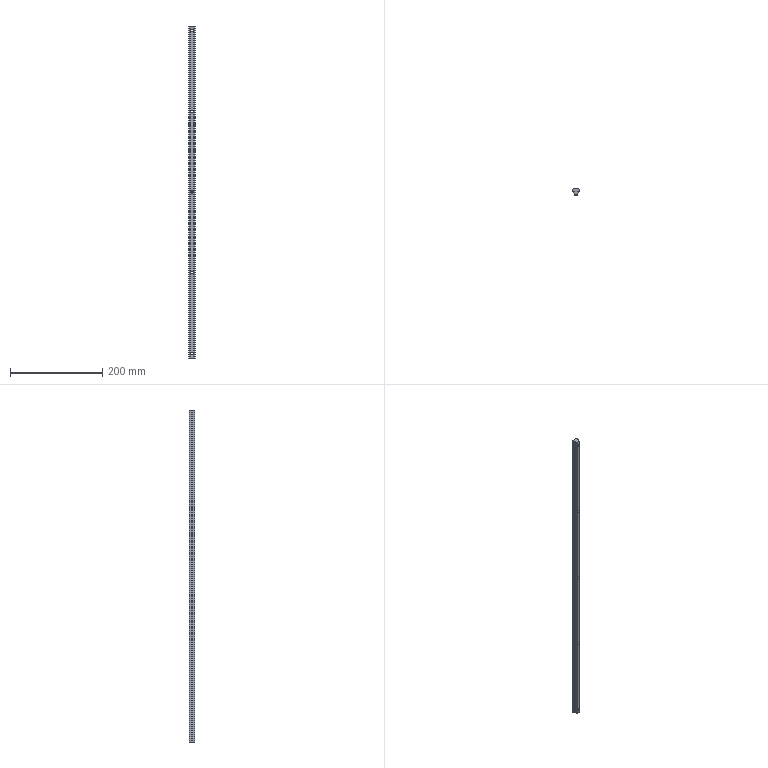Part | STEP file | TJ-DHQM-003-017 | 1 solid | 39 faces | box 15 x 13 x 720 mm | volume 103094 mm3 | cylinder 20 | plane 19 | commonest cylinder face diameters 5.5 x10 10 x10
STEP:
#1=CARTESIAN_POINT('',(0.,7.3,705.));
#2=VERTEX_POINT('',#1);
#3=CARTESIAN_POINT('',(0.,7.3,715.));
#4=VERTEX_POINT('',#3);
#5=CARTESIAN_POINT('',(0.,7.3,710.));
#6=DIRECTION('',(0.,1.,0.));
#7=DIRECTION('',(0.,0.,1.));
#8=AXIS2_PLACEMENT_3D('',#5,#6,#7);
#9=CIRCLE('',#8,5.);
#10=EDGE_CURVE('',#2,#4,#9,.T.);
#11=ORIENTED_EDGE('',*,*,#10,.F.);
#12=CARTESIAN_POINT('',(0.,13.,705.));
#13=VERTEX_POINT('',#12);
#14=CARTESIAN_POINT('',(0.,13.,705.));
#15=DIRECTION('',(0.,1.,0.));
#16=VECTOR('',#15,1000.);
#17=LINE('',#14,#16);
#18=EDGE_CURVE('',#2,#13,#17,.T.);
#19=ORIENTED_EDGE('',*,*,#18,.T.);
#20=CARTESIAN_POINT('',(0.,13.,715.));
#21=VERTEX_POINT('',#20);
#22=CARTESIAN_POINT('',(0.,13.,710.));
#23=DIRECTION('',(0.,1.,0.));
#24=DIRECTION('',(0.,0.,1.));
#25=AXIS2_PLACEMENT_3D('',#22,#23,#24);
#26=CIRCLE('',#25,5.);
#27=EDGE_CURVE('',#13,#21,#26,.T.);
#28=ORIENTED_EDGE('',*,*,#27,.T.);
#29=CARTESIAN_POINT('',(0.,13.,715.));
#30=DIRECTION('',(0.,1.,0.));
#31=VECTOR('',#30,1000.);
#32=LINE('',#29,#31);
#33=EDGE_CURVE('',#4,#21,#32,.T.);
#34=ORIENTED_EDGE('',*,*,#33,.F.);
#35=EDGE_LOOP('',(#11,#19,#28,#34));
#36=FACE_OUTER_BOUND('',#35,.T.);
#37=CARTESIAN_POINT('',(0.,13.,710.));
#38=DIRECTION('',(0.,1.,0.));
#39=DIRECTION('',(0.,0.,1.));
#40=AXIS2_PLACEMENT_3D('',#37,#38,#39);
#41=CYLINDRICAL_SURFACE('',#40,5.);
#42=ADVANCED_FACE('',(#36),#41,.F.);
#43=CARTESIAN_POINT('',(0.,0.,707.25));
#44=VERTEX_POINT('',#43);
#45=CARTESIAN_POINT('',(0.,0.,712.75));
#46=VERTEX_POINT('',#45);
#47=CARTESIAN_POINT('',(0.,0.,710.));
#48=DIRECTION('',(0.,1.,0.));
#49=DIRECTION('',(0.,0.,1.));
#50=AXIS2_PLACEMENT_3D('',#47,#48,#49);
#51=CIRCLE('',#50,2.75);
#52=EDGE_CURVE('',#44,#46,#51,.T.);
#53=ORIENTED_EDGE('',*,*,#52,.F.);
#54=CARTESIAN_POINT('',(0.,7.3,707.25));
#55=VERTEX_POINT('',#54);
#56=CARTESIAN_POINT('',(0.,13.,707.25));
#57=DIRECTION('',(0.,1.,0.));
#58=VECTOR('',#57,1000.);
#59=LINE('',#56,#58);
#60=EDGE_CURVE('',#44,#55,#59,.T.);
#61=ORIENTED_EDGE('',*,*,#60,.T.);
#62=CARTESIAN_POINT('',(0.,7.3,712.75));
#63=VERTEX_POINT('',#62);
#64=CARTESIAN_POINT('',(0.,7.3,710.));
#65=DIRECTION('',(0.,1.,0.));
#66=DIRECTION('',(0.,0.,1.));
#67=AXIS2_PLACEMENT_3D('',#64,#65,#66);
#68=CIRCLE('',#67,2.75);
#69=EDGE_CURVE('',#55,#63,#68,.T.);
#70=ORIENTED_EDGE('',*,*,#69,.T.);
#71=CARTESIAN_POINT('',(0.,13.,712.75));
#72=DIRECTION('',(0.,1.,0.));
#73=VECTOR('',#72,1000.);
#74=LINE('',#71,#73);
#75=EDGE_CURVE('',#46,#63,#74,.T.);
#76=ORIENTED_EDGE('',*,*,#75,.F.);
#77=EDGE_LOOP('',(#53,#61,#70,#76));
#78=FACE_OUTER_BOUND('',#77,.T.);
#79=CARTESIAN_POINT('',(0.,13.,710.));
#80=DIRECTION('',(0.,1.,0.));
#81=DIRECTION('',(0.,0.,1.));
#82=AXIS2_PLACEMENT_3D('',#79,#80,#81);
#83=CYLINDRICAL_SURFACE('',#82,2.75);
#84=ADVANCED_FACE('',(#78),#83,.F.);
#85=CARTESIAN_POINT('',(0.,7.3,355.));
#86=VERTEX_POINT('',#85);
#87=CARTESIAN_POINT('',(0.,7.3,365.));
#88=VERTEX_POINT('',#87);
#89=CARTESIAN_POINT('',(0.,7.3,360.));
#90=DIRECTION('',(0.,1.,0.));
#91=DIRECTION('',(0.,0.,1.));
#92=AXIS2_PLACEMENT_3D('',#89,#90,#91);
#93=CIRCLE('',#92,5.);
#94=EDGE_CURVE('',#86,#88,#93,.T.);
#95=ORIENTED_EDGE('',*,*,#94,.F.);
#96=CARTESIAN_POINT('',(0.,13.,355.));
#97=VERTEX_POINT('',#96);
#98=CARTESIAN_POINT('',(0.,13.,355.));
#99=DIRECTION('',(0.,1.,0.));
#100=VECTOR('',#99,1000.);
#101=LINE('',#98,#100);
#102=EDGE_CURVE('',#86,#97,#101,.T.);
#103=ORIENTED_EDGE('',*,*,#102,.T.);
#104=CARTESIAN_POINT('',(0.,13.,365.));
#105=VERTEX_POINT('',#104);
#106=CARTESIAN_POINT('',(0.,13.,360.));
#107=DIRECTION('',(0.,1.,0.));
#108=DIRECTION('',(0.,0.,1.));
#109=AXIS2_PLACEMENT_3D('',#106,#107,#108);
#110=CIRCLE('',#109,5.);
#111=EDGE_CURVE('',#97,#105,#110,.T.);
#112=ORIENTED_EDGE('',*,*,#111,.T.);
#113=CARTESIAN_POINT('',(0.,13.,365.));
#114=DIRECTION('',(0.,1.,0.));
#115=VECTOR('',#114,1000.);
#116=LINE('',#113,#115);
#117=EDGE_CURVE('',#88,#105,#116,.T.);
#118=ORIENTED_EDGE('',*,*,#117,.F.);
#119=EDGE_LOOP('',(#95,#103,#112,#118));
#120=FACE_OUTER_BOUND('',#119,.T.);
#121=CARTESIAN_POINT('',(0.,13.,360.));
#122=DIRECTION('',(0.,1.,0.));
#123=DIRECTION('',(0.,0.,1.));
#124=AXIS2_PLACEMENT_3D('',#121,#122,#123);
#125=CYLINDRICAL_SURFACE('',#124,5.);
#126=ADVANCED_FACE('',(#120),#125,.F.);
#127=CARTESIAN_POINT('',(0.,0.,357.25));
#128=VERTEX_POINT('',#127);
#129=CARTESIAN_POINT('',(0.,0.,362.75));
#130=VERTEX_POINT('',#129);
#131=CARTESIAN_POINT('',(0.,0.,360.));
#132=DIRECTION('',(0.,1.,0.));
#133=DIRECTION('',(0.,0.,1.));
#134=AXIS2_PLACEMENT_3D('',#131,#132,#133);
#135=CIRCLE('',#134,2.75);
#136=EDGE_CURVE('',#128,#130,#135,.T.);
#137=ORIENTED_EDGE('',*,*,#136,.F.);
#138=CARTESIAN_POINT('',(0.,7.3,357.25));
#139=VERTEX_POINT('',#138);
#140=CARTESIAN_POINT('',(0.,13.,357.25));
#141=DIRECTION('',(0.,1.,0.));
#142=VECTOR('',#141,1000.);
#143=LINE('',#140,#142);
#144=EDGE_CURVE('',#128,#139,#143,.T.);
#145=ORIENTED_EDGE('',*,*,#144,.T.);
#146=CARTESIAN_POINT('',(0.,7.3,362.75));
#147=VERTEX_POINT('',#146);
#148=CARTESIAN_POINT('',(0.,7.3,360.));
#149=DIRECTION('',(0.,1.,0.));
#150=DIRECTION('',(0.,0.,1.));
#151=AXIS2_PLACEMENT_3D('',#148,#149,#150);
#152=CIRCLE('',#151,2.75);
#153=EDGE_CURVE('',#139,#147,#152,.T.);
#154=ORIENTED_EDGE('',*,*,#153,.T.);
#155=CARTESIAN_POINT('',(0.,13.,362.75));
#156=DIRECTION('',(0.,1.,0.));
#157=VECTOR('',#156,1000.);
#158=LINE('',#155,#157);
#159=EDGE_CURVE('',#130,#147,#158,.T.);
#160=ORIENTED_EDGE('',*,*,#159,.F.);
#161=EDGE_LOOP('',(#137,#145,#154,#160));
#162=FACE_OUTER_BOUND('',#161,.T.);
#163=CARTESIAN_POINT('',(0.,13.,360.));
#164=DIRECTION('',(0.,1.,0.));
#165=DIRECTION('',(0.,0.,1.));
#166=AXIS2_PLACEMENT_3D('',#163,#164,#165);
#167=CYLINDRICAL_SURFACE('',#166,2.75);
#168=ADVANCED_FACE('',(#162),#167,.F.);
#169=CARTESIAN_POINT('',(0.,7.3,530.));
#170=VERTEX_POINT('',#169);
#171=CARTESIAN_POINT('',(0.,7.3,540.));
#172=VERTEX_POINT('',#171);
#173=CARTESIAN_POINT('',(0.,7.3,535.));
#174=DIRECTION('',(0.,1.,0.));
#175=DIRECTION('',(0.,0.,1.));
#176=AXIS2_PLACEMENT_3D('',#173,#174,#175);
#177=CIRCLE('',#176,5.);
#178=EDGE_CURVE('',#170,#172,#177,.T.);
#179=ORIENTED_EDGE('',*,*,#178,.F.);
#180=CARTESIAN_POINT('',(0.,13.,530.));
#181=VERTEX_POINT('',#180);
#182=CARTESIAN_POINT('',(0.,13.,530.));
#183=DIRECTION('',(0.,1.,0.));
#184=VECTOR('',#183,1000.);
#185=LINE('',#182,#184);
#186=EDGE_CURVE('',#170,#181,#185,.T.);
#187=ORIENTED_EDGE('',*,*,#186,.T.);
#188=CARTESIAN_POINT('',(0.,13.,540.));
#189=VERTEX_POINT('',#188);
#190=CARTESIAN_POINT('',(0.,13.,535.));
#191=DIRECTION('',(0.,1.,0.));
#192=DIRECTION('',(0.,0.,1.));
#193=AXIS2_PLACEMENT_3D('',#190,#191,#192);
#194=CIRCLE('',#193,5.);
#195=EDGE_CURVE('',#181,#189,#194,.T.);
#196=ORIENTED_EDGE('',*,*,#195,.T.);
#197=CARTESIAN_POINT('',(0.,13.,540.));
#198=DIRECTION('',(0.,1.,0.));
#199=VECTOR('',#198,1000.);
#200=LINE('',#197,#199);
#201=EDGE_CURVE('',#172,#189,#200,.T.);
#202=ORIENTED_EDGE('',*,*,#201,.F.);
#203=EDGE_LOOP('',(#179,#187,#196,#202));
#204=FACE_OUTER_BOUND('',#203,.T.);
#205=CARTESIAN_POINT('',(0.,13.,535.));
#206=DIRECTION('',(0.,1.,0.));
#207=DIRECTION('',(0.,0.,1.));
#208=AXIS2_PLACEMENT_3D('',#205,#206,#207);
#209=CYLINDRICAL_SURFACE('',#208,5.);
#210=ADVANCED_FACE('',(#204),#209,.F.);
#211=CARTESIAN_POINT('',(0.,0.,532.25));
#212=VERTEX_POINT('',#211);
#213=CARTESIAN_POINT('',(0.,0.,537.75));
#214=VERTEX_POINT('',#213);
#215=CARTESIAN_POINT('',(0.,0.,535.));
#216=DIRECTION('',(0.,1.,0.));
#217=DIRECTION('',(0.,0.,1.));
#218=AXIS2_PLACEMENT_3D('',#215,#216,#217);
#219=CIRCLE('',#218,2.75);
#220=EDGE_CURVE('',#212,#214,#219,.T.);
#221=ORIENTED_EDGE('',*,*,#220,.F.);
#222=CARTESIAN_POINT('',(0.,7.3,532.25));
#223=VERTEX_POINT('',#222);
#224=CARTESIAN_POINT('',(0.,13.,532.25));
#225=DIRECTION('',(0.,1.,0.));
#226=VECTOR('',#225,1000.);
#227=LINE('',#224,#226);
#228=EDGE_CURVE('',#212,#223,#227,.T.);
#229=ORIENTED_EDGE('',*,*,#228,.T.);
#230=CARTESIAN_POINT('',(0.,7.3,537.75));
#231=VERTEX_POINT('',#230);
#232=CARTESIAN_POINT('',(0.,7.3,535.));
#233=DIRECTION('',(0.,1.,0.));
#234=DIRECTION('',(0.,0.,1.));
#235=AXIS2_PLACEMENT_3D('',#232,#233,#234);
#236=CIRCLE('',#235,2.75);
#237=EDGE_CURVE('',#223,#231,#236,.T.);
#238=ORIENTED_EDGE('',*,*,#237,.T.);
#239=CARTESIAN_POINT('',(0.,13.,537.75));
#240=DIRECTION('',(0.,1.,0.));
#241=VECTOR('',#240,1000.);
#242=LINE('',#239,#241);
#243=EDGE_CURVE('',#214,#231,#242,.T.);
#244=ORIENTED_EDGE('',*,*,#243,.F.);
#245=EDGE_LOOP('',(#221,#229,#238,#244));
#246=FACE_OUTER_BOUND('',#245,.T.);
#247=CARTESIAN_POINT('',(0.,13.,535.));
#248=DIRECTION('',(0.,1.,0.));
#249=DIRECTION('',(0.,0.,1.));
#250=AXIS2_PLACEMENT_3D('',#247,#248,#249);
#251=CYLINDRICAL_SURFACE('',#250,2.75);
#252=ADVANCED_FACE('',(#246),#251,.F.);
#253=CARTESIAN_POINT('',(0.,7.3,180.));
#254=VERTEX_POINT('',#253);
#255=CARTESIAN_POINT('',(0.,7.3,190.));
#256=VERTEX_POINT('',#255);
#257=CARTESIAN_POINT('',(0.,7.3,185.));
#258=DIRECTION('',(0.,1.,0.));
#259=DIRECTION('',(0.,0.,1.));
#260=AXIS2_PLACEMENT_3D('',#257,#258,#259);
#261=CIRCLE('',#260,5.);
#262=EDGE_CURVE('',#254,#256,#261,.T.);
#263=ORIENTED_EDGE('',*,*,#262,.F.);
#264=CARTESIAN_POINT('',(0.,13.,180.));
#265=VERTEX_POINT('',#264);
#266=CARTESIAN_POINT('',(0.,13.,180.));
#267=DIRECTION('',(0.,1.,0.));
#268=VECTOR('',#267,1000.);
#269=LINE('',#266,#268);
#270=EDGE_CURVE('',#254,#265,#269,.T.);
#271=ORIENTED_EDGE('',*,*,#270,.T.);
#272=CARTESIAN_POINT('',(0.,13.,190.));
#273=VERTEX_POINT('',#272);
#274=CARTESIAN_POINT('',(0.,13.,185.));
#275=DIRECTION('',(0.,1.,0.));
#276=DIRECTION('',(0.,0.,1.));
#277=AXIS2_PLACEMENT_3D('',#274,#275,#276);
#278=CIRCLE('',#277,5.);
#279=EDGE_CURVE('',#265,#273,#278,.T.);
#280=ORIENTED_EDGE('',*,*,#279,.T.);
#281=CARTESIAN_POINT('',(0.,13.,190.));
#282=DIRECTION('',(0.,1.,0.));
#283=VECTOR('',#282,1000.);
#284=LINE('',#281,#283);
#285=EDGE_CURVE('',#256,#273,#284,.T.);
#286=ORIENTED_EDGE('',*,*,#285,.F.);
#287=EDGE_LOOP('',(#263,#271,#280,#286));
#288=FACE_OUTER_BOUND('',#287,.T.);
#289=CARTESIAN_POINT('',(0.,13.,185.));
#290=DIRECTION('',(0.,1.,0.));
#291=DIRECTION('',(0.,0.,1.));
#292=AXIS2_PLACEMENT_3D('',#289,#290,#291);
#293=CYLINDRICAL_SURFACE('',#292,5.);
#294=ADVANCED_FACE('',(#288),#293,.F.);
#295=CARTESIAN_POINT('',(0.,0.,182.25));
#296=VERTEX_POINT('',#295);
#297=CARTESIAN_POINT('',(0.,0.,187.75));
#298=VERTEX_POINT('',#297);
#299=CARTESIAN_POINT('',(0.,0.,185.));
#300=DIRECTION('',(0.,1.,0.));
#301=DIRECTION('',(0.,0.,1.));
#302=AXIS2_PLACEMENT_3D('',#299,#300,#301);
#303=CIRCLE('',#302,2.75);
#304=EDGE_CURVE('',#296,#298,#303,.T.);
#305=ORIENTED_EDGE('',*,*,#304,.F.);
#306=CARTESIAN_POINT('',(0.,7.3,182.25));
#307=VERTEX_POINT('',#306);
#308=CARTESIAN_POINT('',(0.,13.,182.25));
#309=DIRECTION('',(0.,1.,0.));
#310=VECTOR('',#309,1000.);
#311=LINE('',#308,#310);
#312=EDGE_CURVE('',#296,#307,#311,.T.);
#313=ORIENTED_EDGE('',*,*,#312,.T.);
#314=CARTESIAN_POINT('',(0.,7.3,187.75));
#315=VERTEX_POINT('',#314);
#316=CARTESIAN_POINT('',(0.,7.3,185.));
#317=DIRECTION('',(0.,1.,0.));
#318=DIRECTION('',(0.,0.,1.));
#319=AXIS2_PLACEMENT_3D('',#316,#317,#318);
#320=CIRCLE('',#319,2.75);
#321=EDGE_CURVE('',#307,#315,#320,.T.);
#322=ORIENTED_EDGE('',*,*,#321,.T.);
#323=CARTESIAN_POINT('',(0.,13.,187.75));
#324=DIRECTION('',(0.,1.,0.));
#325=VECTOR('',#324,1000.);
#326=LINE('',#323,#325);
#327=EDGE_CURVE('',#298,#315,#326,.T.);
#328=ORIENTED_EDGE('',*,*,#327,.F.);
#329=EDGE_LOOP('',(#305,#313,#322,#328));
#330=FACE_OUTER_BOUND('',#329,.T.);
#331=CARTESIAN_POINT('',(0.,13.,185.));
#332=DIRECTION('',(0.,1.,0.));
#333=DIRECTION('',(0.,0.,1.));
#334=AXIS2_PLACEMENT_3D('',#331,#332,#333);
#335=CYLINDRICAL_SURFACE('',#334,2.75);
#336=ADVANCED_FACE('',(#330),#335,.F.);
#337=CARTESIAN_POINT('',(0.,7.3,5.));
#338=VERTEX_POINT('',#337);
#339=CARTESIAN_POINT('',(0.,7.3,15.));
#340=VERTEX_POINT('',#339);
#341=CARTESIAN_POINT('',(0.,7.3,10.));
#342=DIRECTION('',(0.,1.,0.));
#343=DIRECTION('',(0.,0.,1.));
#344=AXIS2_PLACEMENT_3D('',#341,#342,#343);
#345=CIRCLE('',#344,5.);
#346=EDGE_CURVE('',#338,#340,#345,.T.);
#347=ORIENTED_EDGE('',*,*,#346,.F.);
#348=CARTESIAN_POINT('',(0.,13.,5.));
#349=VERTEX_POINT('',#348);
#350=CARTESIAN_POINT('',(0.,13.,5.));
#351=DIRECTION('',(0.,1.,0.));
#352=VECTOR('',#351,1000.);
#353=LINE('',#350,#352);
#354=EDGE_CURVE('',#338,#349,#353,.T.);
#355=ORIENTED_EDGE('',*,*,#354,.T.);
#356=CARTESIAN_POINT('',(0.,13.,15.));
#357=VERTEX_POINT('',#356);
#358=CARTESIAN_POINT('',(0.,13.,10.));
#359=DIRECTION('',(0.,1.,0.));
#360=DIRECTION('',(0.,0.,1.));
#361=AXIS2_PLACEMENT_3D('',#358,#359,#360);
#362=CIRCLE('',#361,5.);
#363=EDGE_CURVE('',#349,#357,#362,.T.);
#364=ORIENTED_EDGE('',*,*,#363,.T.);
#365=CARTESIAN_POINT('',(0.,13.,15.));
#366=DIRECTION('',(0.,1.,0.));
#367=VECTOR('',#366,1000.);
#368=LINE('',#365,#367);
#369=EDGE_CURVE('',#340,#357,#368,.T.);
#370=ORIENTED_EDGE('',*,*,#369,.F.);
#371=EDGE_LOOP('',(#347,#355,#364,#370));
#372=FACE_OUTER_BOUND('',#371,.T.);
#373=CARTESIAN_POINT('',(0.,13.,10.));
#374=DIRECTION('',(0.,1.,0.));
#375=DIRECTION('',(0.,0.,1.));
#376=AXIS2_PLACEMENT_3D('',#373,#374,#375);
#377=CYLINDRICAL_SURFACE('',#376,5.);
#378=ADVANCED_FACE('',(#372),#377,.F.);
#379=CARTESIAN_POINT('',(0.,0.,7.25));
#380=VERTEX_POINT('',#379);
#381=CARTESIAN_POINT('',(0.,0.,12.75));
#382=VERTEX_POINT('',#381);
#383=CARTESIAN_POINT('',(0.,0.,10.));
#384=DIRECTION('',(0.,1.,0.));
#385=DIRECTION('',(0.,0.,1.));
#386=AXIS2_PLACEMENT_3D('',#383,#384,#385);
#387=CIRCLE('',#386,2.75);
#388=EDGE_CURVE('',#380,#382,#387,.T.);
#389=ORIENTED_EDGE('',*,*,#388,.F.);
#390=CARTESIAN_POINT('',(0.,7.3,7.25));
#391=VERTEX_POINT('',#390);
#392=CARTESIAN_POINT('',(0.,13.,7.25));
#393=DIRECTION('',(0.,1.,0.));
#394=VECTOR('',#393,1000.);
#395=LINE('',#392,#394);
#396=EDGE_CURVE('',#380,#391,#395,.T.);
#397=ORIENTED_EDGE('',*,*,#396,.T.);
#398=CARTESIAN_POINT('',(0.,7.3,12.75));
#399=VERTEX_POINT('',#398);
#400=CARTESIAN_POINT('',(0.,7.3,10.));
#401=DIRECTION('',(0.,1.,0.));
#402=DIRECTION('',(0.,0.,1.));
#403=AXIS2_PLACEMENT_3D('',#400,#401,#402);
#404=CIRCLE('',#403,2.75);
#405=EDGE_CURVE('',#391,#399,#404,.T.);
#406=ORIENTED_EDGE('',*,*,#405,.T.);
#407=CARTESIAN_POINT('',(0.,13.,12.75));
#408=DIRECTION('',(0.,1.,0.));
#409=VECTOR('',#408,1000.);
#410=LINE('',#407,#409);
#411=EDGE_CURVE('',#382,#399,#410,.T.);
#412=ORIENTED_EDGE('',*,*,#411,.F.);
#413=EDGE_LOOP('',(#389,#397,#406,#412));
#414=FACE_OUTER_BOUND('',#413,.T.);
#415=CARTESIAN_POINT('',(0.,13.,10.));
#416=DIRECTION('',(0.,1.,0.));
#417=DIRECTION('',(0.,0.,1.));
#418=AXIS2_PLACEMENT_3D('',#415,#416,#417);
#419=CYLINDRICAL_SURFACE('',#418,2.75);
#420=ADVANCED_FACE('',(#414),#419,.F.);
#421=CARTESIAN_POINT('',(7.5,7.5,720.));
#422=VERTEX_POINT('',#421);
#423=CARTESIAN_POINT('',(7.5,12.,720.));
#424=VERTEX_POINT('',#423);
#425=CARTESIAN_POINT('',(7.5,13.,720.));
#426=DIRECTION('',(0.,1.,0.));
#427=VECTOR('',#426,1000.);
#428=LINE('',#425,#427);
#429=EDGE_CURVE('',#422,#424,#428,.T.);
#430=ORIENTED_EDGE('',*,*,#429,.F.);
#431=CARTESIAN_POINT('',(7.5,7.5,0.));
#432=VERTEX_POINT('',#431);
#433=CARTESIAN_POINT('',(7.5,7.5,720.));
#434=DIRECTION('',(0.,0.,-1.));
#435=VECTOR('',#434,1000.);
#436=LINE('',#433,#435);
#437=EDGE_CURVE('',#422,#432,#436,.T.);
#438=ORIENTED_EDGE('',*,*,#437,.T.);
#439=CARTESIAN_POINT('',(7.5,12.,0.));
#440=VERTEX_POINT('',#439);
#441=CARTESIAN_POINT('',(7.5,13.,0.));
#442=DIRECTION('',(0.,1.,0.));
#443=VECTOR('',#442,1000.);
#444=LINE('',#441,#443);
#445=EDGE_CURVE('',#432,#440,#444,.T.);
#446=ORIENTED_EDGE('',*,*,#445,.T.);
#447=CARTESIAN_POINT('',(7.5,12.,720.));
#448=DIRECTION('',(0.,0.,1.));
#449=VECTOR('',#448,1000.);
#450=LINE('',#447,#449);
#451=EDGE_CURVE('',#440,#424,#450,.T.);
#452=ORIENTED_EDGE('',*,*,#451,.T.);
#453=EDGE_LOOP('',(#430,#438,#446,#452));
#454=FACE_OUTER_BOUND('',#453,.T.);
#455=CARTESIAN_POINT('',(7.5,13.,720.));
#456=DIRECTION('',(-1.,0.,0.));
#457=DIRECTION('',(0.,-1.,0.));
#458=AXIS2_PLACEMENT_3D('',#455,#456,#457);
#459=PLANE('',#458);
#460=ADVANCED_FACE('',(#454),#459,.F.);
#461=CARTESIAN_POINT('',(0.,13.,710.));
#462=DIRECTION('',(0.,1.,0.));
#463=DIRECTION('',(0.,0.,1.));
#464=AXIS2_PLACEMENT_3D('',#461,#462,#463);
#465=CIRCLE('',#464,5.);
#466=EDGE_CURVE('',#21,#13,#465,.T.);
#467=ORIENTED_EDGE('',*,*,#466,.F.);
#468=ORIENTED_EDGE('',*,*,#27,.F.);
#469=EDGE_LOOP('',(#467,#468));
#470=FACE_BOUND('',#469,.T.);
#471=CARTESIAN_POINT('',(0.,13.,360.));
#472=DIRECTION('',(0.,1.,0.));
#473=DIRECTION('',(0.,0.,1.));
#474=AXIS2_PLACEMENT_3D('',#471,#472,#473);
#475=CIRCLE('',#474,5.);
#476=EDGE_CURVE('',#105,#97,#475,.T.);
#477=ORIENTED_EDGE('',*,*,#476,.F.);
#478=ORIENTED_EDGE('',*,*,#111,.F.);
#479=EDGE_LOOP('',(#477,#478));
#480=FACE_BOUND('',#479,.T.);
#481=CARTESIAN_POINT('',(0.,13.,535.));
#482=DIRECTION('',(0.,1.,0.));
#483=DIRECTION('',(0.,0.,1.));
#484=AXIS2_PLACEMENT_3D('',#481,#482,#483);
#485=CIRCLE('',#484,5.);
#486=EDGE_CURVE('',#189,#181,#485,.T.);
#487=ORIENTED_EDGE('',*,*,#486,.F.);
#488=ORIENTED_EDGE('',*,*,#195,.F.);
#489=EDGE_LOOP('',(#487,#488));
#490=FACE_BOUND('',#489,.T.);
#491=CARTESIAN_POINT('',(0.,13.,185.));
#492=DIRECTION('',(0.,1.,0.));
#493=DIRECTION('',(0.,0.,1.));
#494=AXIS2_PLACEMENT_3D('',#491,#492,#493);
#495=CIRCLE('',#494,5.);
#496=EDGE_CURVE('',#273,#265,#495,.T.);
#497=ORIENTED_EDGE('',*,*,#496,.F.);
#498=ORIENTED_EDGE('',*,*,#279,.F.);
#499=EDGE_LOOP('',(#497,#498));
#500=FACE_BOUND('',#499,.T.);
#501=CARTESIAN_POINT('',(0.,13.,10.));
#502=DIRECTION('',(0.,1.,0.));
#503=DIRECTION('',(0.,0.,1.));
#504=AXIS2_PLACEMENT_3D('',#501,#502,#503);
#505=CIRCLE('',#504,5.);
#506=EDGE_CURVE('',#357,#349,#505,.T.);
#507=ORIENTED_EDGE('',*,*,#506,.F.);
#508=ORIENTED_EDGE('',*,*,#363,.F.);
#509=EDGE_LOOP('',(#507,#508));
#510=FACE_BOUND('',#509,.T.);
#511=CARTESIAN_POINT('',(6.5,13.,0.));
#512=VERTEX_POINT('',#511);
#513=CARTESIAN_POINT('',(-6.5,13.,0.));
#514=VERTEX_POINT('',#513);
#515=CARTESIAN_POINT('',(-7.5,13.,0.));
#516=DIRECTION('',(-1.,0.,0.));
#517=VECTOR('',#516,1000.);
#518=LINE('',#515,#517);
#519=EDGE_CURVE('',#512,#514,#518,.T.);
#520=ORIENTED_EDGE('',*,*,#519,.T.);
#521=CARTESIAN_POINT('',(-6.5,13.,720.));
#522=VERTEX_POINT('',#521);
#523=CARTESIAN_POINT('',(-6.5,13.,720.));
#524=DIRECTION('',(0.,0.,1.));
#525=VECTOR('',#524,1000.);
#526=LINE('',#523,#525);
#527=EDGE_CURVE('',#514,#522,#526,.T.);
#528=ORIENTED_EDGE('',*,*,#527,.T.);
#529=CARTESIAN_POINT('',(6.5,13.,720.));
#530=VERTEX_POINT('',#529);
#531=CARTESIAN_POINT('',(-7.5,13.,720.));
#532=DIRECTION('',(-1.,0.,0.));
#533=VECTOR('',#532,1000.);
#534=LINE('',#531,#533);
#535=EDGE_CURVE('',#530,#522,#534,.T.);
#536=ORIENTED_EDGE('',*,*,#535,.F.);
#537=CARTESIAN_POINT('',(6.5,13.,720.));
#538=DIRECTION('',(0.,0.,-1.));
#539=VECTOR('',#538,1000.);
#540=LINE('',#537,#539);
#541=EDGE_CURVE('',#530,#512,#540,.T.);
#542=ORIENTED_EDGE('',*,*,#541,.T.);
#543=EDGE_LOOP('',(#520,#528,#536,#542));
#544=FACE_OUTER_BOUND('',#543,.T.);
#545=CARTESIAN_POINT('',(-7.5,13.,720.));
#546=DIRECTION('',(0.,-1.,0.));
#547=DIRECTION('',(0.,0.,-1.));
#548=AXIS2_PLACEMENT_3D('',#545,#546,#547);
#549=PLANE('',#548);
#550=ADVANCED_FACE('',(#470,#480,#490,#500,#510,#544),#549,.F.);
#551=CARTESIAN_POINT('',(-7.5,12.,0.));
#552=VERTEX_POINT('',#551);
#553=CARTESIAN_POINT('',(-7.5,7.5,0.));
#554=VERTEX_POINT('',#553);
#555=CARTESIAN_POINT('',(-7.5,13.,0.));
#556=DIRECTION('',(0.,-1.,0.));
#557=VECTOR('',#556,1000.);
#558=LINE('',#555,#557);
#559=EDGE_CURVE('',#552,#554,#558,.T.);
#560=ORIENTED_EDGE('',*,*,#559,.T.);
#561=CARTESIAN_POINT('',(-7.5,7.5,720.));
#562=VERTEX_POINT('',#561);
#563=CARTESIAN_POINT('',(-7.5,7.5,720.));
#564=DIRECTION('',(0.,0.,1.));
#565=VECTOR('',#564,1000.);
#566=LINE('',#563,#565);
#567=EDGE_CURVE('',#554,#562,#566,.T.);
#568=ORIENTED_EDGE('',*,*,#567,.T.);
#569=CARTESIAN_POINT('',(-7.5,12.,720.));
#570=VERTEX_POINT('',#569);
#571=CARTESIAN_POINT('',(-7.5,13.,720.));
#572=DIRECTION('',(0.,-1.,0.));
#573=VECTOR('',#572,1000.);
#574=LINE('',#571,#573);
#575=EDGE_CURVE('',#570,#562,#574,.T.);
#576=ORIENTED_EDGE('',*,*,#575,.F.);
#577=CARTESIAN_POINT('',(-7.5,12.,720.));
#578=DIRECTION('',(0.,0.,-1.));
#579=VECTOR('',#578,1000.);
#580=LINE('',#577,#579);
#581=EDGE_CURVE('',#570,#552,#580,.T.);
#582=ORIENTED_EDGE('',*,*,#581,.T.);
#583=EDGE_LOOP('',(#560,#568,#576,#582));
#584=FACE_OUTER_BOUND('',#583,.T.);
#585=CARTESIAN_POINT('',(-7.5,13.,720.));
#586=DIRECTION('',(1.,0.,0.));
#587=DIRECTION('',(0.,1.,0.));
#588=AXIS2_PLACEMENT_3D('',#585,#586,#587);
#589=PLANE('',#588);
#590=ADVANCED_FACE('',(#584),#589,.F.);
#591=CARTESIAN_POINT('',(-6.5,6.5,720.));
#592=VERTEX_POINT('',#591);
#593=CARTESIAN_POINT('',(-4.,6.5,720.));
#594=VERTEX_POINT('',#593);
#595=CARTESIAN_POINT('',(-7.5,6.5,720.));
#596=DIRECTION('',(1.,0.,0.));
#597=VECTOR('',#596,1000.);
#598=LINE('',#595,#597);
#599=EDGE_CURVE('',#592,#594,#598,.T.);
#600=ORIENTED_EDGE('',*,*,#599,.F.);
#601=CARTESIAN_POINT('',(-6.5,6.5,0.));
#602=VERTEX_POINT('',#601);
#603=CARTESIAN_POINT('',(-6.5,6.5,720.));
#604=DIRECTION('',(0.,0.,-1.));
#605=VECTOR('',#604,1000.);
#606=LINE('',#603,#605);
#607=EDGE_CURVE('',#592,#602,#606,.T.);
#608=ORIENTED_EDGE('',*,*,#607,.T.);
#609=CARTESIAN_POINT('',(-4.,6.5,0.));
#610=VERTEX_POINT('',#609);
#611=CARTESIAN_POINT('',(-7.5,6.5,0.));
#612=DIRECTION('',(1.,0.,0.));
#613=VECTOR('',#612,1000.);
#614=LINE('',#611,#613);
#615=EDGE_CURVE('',#602,#610,#614,.T.);
#616=ORIENTED_EDGE('',*,*,#615,.T.);
#617=CARTESIAN_POINT('',(-4.,6.5,720.));
#618=DIRECTION('',(0.,0.,-1.));
#619=VECTOR('',#618,1000.);
#620=LINE('',#617,#619);
#621=EDGE_CURVE('',#594,#610,#620,.T.);
#622=ORIENTED_EDGE('',*,*,#621,.F.);
#623=EDGE_LOOP('',(#600,#608,#616,#622));
#624=FACE_OUTER_BOUND('',#623,.T.);
#625=CARTESIAN_POINT('',(-7.5,6.5,720.));
#626=DIRECTION('',(0.,1.,0.));
#627=DIRECTION('',(0.,0.,1.));
#628=AXIS2_PLACEMENT_3D('',#625,#626,#627);
#629=PLANE('',#628);
#630=ADVANCED_FACE('',(#624),#629,.F.);
#631=CARTESIAN_POINT('',(-4.,0.,0.));
#632=VERTEX_POINT('',#631);
#633=CARTESIAN_POINT('',(-4.,6.5,0.));
#634=DIRECTION('',(0.,-1.,0.));
#635=VECTOR('',#634,1000.);
#636=LINE('',#633,#635);
#637=EDGE_CURVE('',#610,#632,#636,.T.);
#638=ORIENTED_EDGE('',*,*,#637,.T.);
#639=CARTESIAN_POINT('',(-4.,0.,720.));
#640=VERTEX_POINT('',#639);
#641=CARTESIAN_POINT('',(-4.,0.,720.));
#642=DIRECTION('',(0.,0.,-1.));
#643=VECTOR('',#642,1000.);
#644=LINE('',#641,#643);
#645=EDGE_CURVE('',#640,#632,#644,.T.);
#646=ORIENTED_EDGE('',*,*,#645,.F.);
#647=CARTESIAN_POINT('',(-4.,6.5,720.));
#648=DIRECTION('',(0.,-1.,0.));
#649=VECTOR('',#648,1000.);
#650=LINE('',#647,#649);
#651=EDGE_CURVE('',#594,#640,#650,.T.);
#652=ORIENTED_EDGE('',*,*,#651,.F.);
#653=ORIENTED_EDGE('',*,*,#621,.T.);
#654=EDGE_LOOP('',(#638,#646,#652,#653));
#655=FACE_OUTER_BOUND('',#654,.T.);
#656=CARTESIAN_POINT('',(-4.,6.5,720.));
#657=DIRECTION('',(1.,0.,0.));
#658=DIRECTION('',(0.,1.,0.));
#659=AXIS2_PLACEMENT_3D('',#656,#657,#658);
#660=PLANE('',#659);
#661=ADVANCED_FACE('',(#655),#660,.F.);
#662=CARTESIAN_POINT('',(0.,0.,710.));
#663=DIRECTION('',(0.,1.,0.));
#664=DIRECTION('',(0.,0.,1.));
#665=AXIS2_PLACEMENT_3D('',#662,#663,#664);
#666=CIRCLE('',#665,2.75);
#667=EDGE_CURVE('',#46,#44,#666,.T.);
#668=ORIENTED_EDGE('',*,*,#667,.T.);
#669=ORIENTED_EDGE('',*,*,#52,.T.);
#670=EDGE_LOOP('',(#668,#669));
#671=FACE_BOUND('',#670,.T.);
#672=CARTESIAN_POINT('',(0.,0.,360.));
#673=DIRECTION('',(0.,1.,0.));
#674=DIRECTION('',(0.,0.,1.));
#675=AXIS2_PLACEMENT_3D('',#672,#673,#674);
#676=CIRCLE('',#675,2.75);
#677=EDGE_CURVE('',#130,#128,#676,.T.);
#678=ORIENTED_EDGE('',*,*,#677,.T.);
#679=ORIENTED_EDGE('',*,*,#136,.T.);
#680=EDGE_LOOP('',(#678,#679));
#681=FACE_BOUND('',#680,.T.);
#682=CARTESIAN_POINT('',(0.,0.,535.));
#683=DIRECTION('',(0.,1.,0.));
#684=DIRECTION('',(0.,0.,1.));
#685=AXIS2_PLACEMENT_3D('',#682,#683,#684);
#686=CIRCLE('',#685,2.75);
#687=EDGE_CURVE('',#214,#212,#686,.T.);
#688=ORIENTED_EDGE('',*,*,#687,.T.);
#689=ORIENTED_EDGE('',*,*,#220,.T.);
#690=EDGE_LOOP('',(#688,#689));
#691=FACE_BOUND('',#690,.T.);
#692=CARTESIAN_POINT('',(0.,0.,185.));
#693=DIRECTION('',(0.,1.,0.));
#694=DIRECTION('',(0.,0.,1.));
#695=AXIS2_PLACEMENT_3D('',#692,#693,#694);
#696=CIRCLE('',#695,2.75);
#697=EDGE_CURVE('',#298,#296,#696,.T.);
#698=ORIENTED_EDGE('',*,*,#697,.T.);
#699=ORIENTED_EDGE('',*,*,#304,.T.);
#700=EDGE_LOOP('',(#698,#699));
#701=FACE_BOUND('',#700,.T.);
#702=CARTESIAN_POINT('',(0.,0.,10.));
#703=DIRECTION('',(0.,1.,0.));
#704=DIRECTION('',(0.,0.,1.));
#705=AXIS2_PLACEMENT_3D('',#702,#703,#704);
#706=CIRCLE('',#705,2.75);
#707=EDGE_CURVE('',#382,#380,#706,.T.);
#708=ORIENTED_EDGE('',*,*,#707,.T.);
#709=ORIENTED_EDGE('',*,*,#388,.T.);
#710=EDGE_LOOP('',(#708,#709));
#711=FACE_BOUND('',#710,.T.);
#712=CARTESIAN_POINT('',(4.,0.,0.));
#713=VERTEX_POINT('',#712);
#714=CARTESIAN_POINT('',(4.,0.,0.));
#715=DIRECTION('',(1.,0.,0.));
#716=VECTOR('',#715,1000.);
#717=LINE('',#714,#716);
#718=EDGE_CURVE('',#632,#713,#717,.T.);
#719=ORIENTED_EDGE('',*,*,#718,.T.);
#720=CARTESIAN_POINT('',(4.,0.,720.));
#721=VERTEX_POINT('',#720);
#722=CARTESIAN_POINT('',(4.,0.,720.));
#723=DIRECTION('',(0.,0.,-1.));
#724=VECTOR('',#723,1000.);
#725=LINE('',#722,#724);
#726=EDGE_CURVE('',#721,#713,#725,.T.);
#727=ORIENTED_EDGE('',*,*,#726,.F.);
#728=CARTESIAN_POINT('',(4.,0.,720.));
#729=DIRECTION('',(1.,0.,0.));
#730=VECTOR('',#729,1000.);
#731=LINE('',#728,#730);
#732=EDGE_CURVE('',#640,#721,#731,.T.);
#733=ORIENTED_EDGE('',*,*,#732,.F.);
#734=ORIENTED_EDGE('',*,*,#645,.T.);
#735=EDGE_LOOP('',(#719,#727,#733,#734));
#736=FACE_OUTER_BOUND('',#735,.T.);
#737=CARTESIAN_POINT('',(4.,0.,720.));
#738=DIRECTION('',(0.,1.,0.));
#739=DIRECTION('',(0.,0.,1.));
#740=AXIS2_PLACEMENT_3D('',#737,#738,#739);
#741=PLANE('',#740);
#742=ADVANCED_FACE('',(#671,#681,#691,#701,#711,#736),#741,.F.);
#743=CARTESIAN_POINT('',(4.,6.5,0.));
#744=VERTEX_POINT('',#743);
#745=CARTESIAN_POINT('',(4.,6.5,0.));
#746=DIRECTION('',(0.,1.,0.));
#747=VECTOR('',#746,1000.);
#748=LINE('',#745,#747);
#749=EDGE_CURVE('',#713,#744,#748,.T.);
#750=ORIENTED_EDGE('',*,*,#749,.T.);
#751=CARTESIAN_POINT('',(4.,6.5,720.));
#752=VERTEX_POINT('',#751);
#753=CARTESIAN_POINT('',(4.,6.5,720.));
#754=DIRECTION('',(0.,0.,-1.));
#755=VECTOR('',#754,1000.);
#756=LINE('',#753,#755);
#757=EDGE_CURVE('',#752,#744,#756,.T.);
#758=ORIENTED_EDGE('',*,*,#757,.F.);
#759=CARTESIAN_POINT('',(4.,6.5,720.));
#760=DIRECTION('',(0.,1.,0.));
#761=VECTOR('',#760,1000.);
#762=LINE('',#759,#761);
#763=EDGE_CURVE('',#721,#752,#762,.T.);
#764=ORIENTED_EDGE('',*,*,#763,.F.);
#765=ORIENTED_EDGE('',*,*,#726,.T.);
#766=EDGE_LOOP('',(#750,#758,#764,#765));
#767=FACE_OUTER_BOUND('',#766,.T.);
#768=CARTESIAN_POINT('',(4.,6.5,720.));
#769=DIRECTION('',(-1.,0.,0.));
#770=DIRECTION('',(0.,-1.,0.));
#771=AXIS2_PLACEMENT_3D('',#768,#769,#770);
#772=PLANE('',#771);
#773=ADVANCED_FACE('',(#767),#772,.F.);
#774=CARTESIAN_POINT('',(6.5,6.5,0.));
#775=VERTEX_POINT('',#774);
#776=CARTESIAN_POINT('',(7.5,6.5,0.));
#777=DIRECTION('',(1.,0.,0.));
#778=VECTOR('',#777,1000.);
#779=LINE('',#776,#778);
#780=EDGE_CURVE('',#744,#775,#779,.T.);
#781=ORIENTED_EDGE('',*,*,#780,.T.);
#782=CARTESIAN_POINT('',(6.5,6.5,720.));
#783=VERTEX_POINT('',#782);
#784=CARTESIAN_POINT('',(6.5,6.5,720.));
#785=DIRECTION('',(0.,0.,1.));
#786=VECTOR('',#785,1000.);
#787=LINE('',#784,#786);
#788=EDGE_CURVE('',#775,#783,#787,.T.);
#789=ORIENTED_EDGE('',*,*,#788,.T.);
#790=CARTESIAN_POINT('',(7.5,6.5,720.));
#791=DIRECTION('',(1.,0.,0.));
#792=VECTOR('',#791,1000.);
#793=LINE('',#790,#792);
#794=EDGE_CURVE('',#752,#783,#793,.T.);
#795=ORIENTED_EDGE('',*,*,#794,.F.);
#796=ORIENTED_EDGE('',*,*,#757,.T.);
#797=EDGE_LOOP('',(#781,#789,#795,#796));
#798=FACE_OUTER_BOUND('',#797,.T.);
#799=CARTESIAN_POINT('',(7.5,6.5,720.));
#800=DIRECTION('',(0.,1.,0.));
#801=DIRECTION('',(0.,0.,1.));
#802=AXIS2_PLACEMENT_3D('',#799,#800,#801);
#803=PLANE('',#802);
#804=ADVANCED_FACE('',(#798),#803,.F.);
#805=ORIENTED_EDGE('',*,*,#575,.T.);
#806=CARTESIAN_POINT('',(-6.5,6.5,720.));
#807=DIRECTION('',(0.7071,-0.7071,0.));
#808=VECTOR('',#807,1000.);
#809=LINE('',#806,#808);
#810=EDGE_CURVE('',#562,#592,#809,.T.);
#811=ORIENTED_EDGE('',*,*,#810,.T.);
#812=ORIENTED_EDGE('',*,*,#599,.T.);
#813=ORIENTED_EDGE('',*,*,#651,.T.);
#814=ORIENTED_EDGE('',*,*,#732,.T.);
#815=ORIENTED_EDGE('',*,*,#763,.T.);
#816=ORIENTED_EDGE('',*,*,#794,.T.);
#817=CARTESIAN_POINT('',(7.5,7.5,720.));
#818=DIRECTION('',(0.7071,0.7071,0.));
#819=VECTOR('',#818,1000.);
#820=LINE('',#817,#819);
#821=EDGE_CURVE('',#783,#422,#820,.T.);
#822=ORIENTED_EDGE('',*,*,#821,.T.);
#823=ORIENTED_EDGE('',*,*,#429,.T.);
#824=CARTESIAN_POINT('',(6.5,13.,720.));
#825=DIRECTION('',(-0.7071,0.7071,0.));
#826=VECTOR('',#825,1000.);
#827=LINE('',#824,#826);
#828=EDGE_CURVE('',#424,#530,#827,.T.);
#829=ORIENTED_EDGE('',*,*,#828,.T.);
#830=ORIENTED_EDGE('',*,*,#535,.T.);
#831=CARTESIAN_POINT('',(-7.5,12.,720.));
#832=DIRECTION('',(-0.7071,-0.7071,0.));
#833=VECTOR('',#832,1000.);
#834=LINE('',#831,#833);
#835=EDGE_CURVE('',#522,#570,#834,.T.);
#836=ORIENTED_EDGE('',*,*,#835,.T.);
#837=EDGE_LOOP('',(#805,#811,#812,#813,#814,#815,#816,#822,#823,#829,#830,#836));
#838=FACE_OUTER_BOUND('',#837,.T.);
#839=CARTESIAN_POINT('',(0.,0.,720.));
#840=DIRECTION('',(0.,0.,-1.));
#841=DIRECTION('',(-1.,0.,0.));
#842=AXIS2_PLACEMENT_3D('',#839,#840,#841);
#843=PLANE('',#842);
#844=ADVANCED_FACE('',(#838),#843,.F.);
#845=ORIENTED_EDGE('',*,*,#615,.F.);
#846=CARTESIAN_POINT('',(0.,0.,0.));
#847=DIRECTION('',(-0.7071,0.7071,0.));
#848=VECTOR('',#847,1000.);
#849=LINE('',#846,#848);
#850=EDGE_CURVE('',#602,#554,#849,.T.);
#851=ORIENTED_EDGE('',*,*,#850,.T.);
#852=ORIENTED_EDGE('',*,*,#559,.F.);
#853=CARTESIAN_POINT('',(-9.75,9.75,0.));
#854=DIRECTION('',(0.7071,0.7071,0.));
#855=VECTOR('',#854,1000.);
#856=LINE('',#853,#855);
#857=EDGE_CURVE('',#552,#514,#856,.T.);
#858=ORIENTED_EDGE('',*,*,#857,.T.);
#859=ORIENTED_EDGE('',*,*,#519,.F.);
#860=CARTESIAN_POINT('',(9.75,9.75,0.));
#861=DIRECTION('',(0.7071,-0.7071,0.));
#862=VECTOR('',#861,1000.);
#863=LINE('',#860,#862);
#864=EDGE_CURVE('',#512,#440,#863,.T.);
#865=ORIENTED_EDGE('',*,*,#864,.T.);
#866=ORIENTED_EDGE('',*,*,#445,.F.);
#867=CARTESIAN_POINT('',(0.,0.,0.));
#868=DIRECTION('',(-0.7071,-0.7071,0.));
#869=VECTOR('',#868,1000.);
#870=LINE('',#867,#869);
#871=EDGE_CURVE('',#432,#775,#870,.T.);
#872=ORIENTED_EDGE('',*,*,#871,.T.);
#873=ORIENTED_EDGE('',*,*,#780,.F.);
#874=ORIENTED_EDGE('',*,*,#749,.F.);
#875=ORIENTED_EDGE('',*,*,#718,.F.);
#876=ORIENTED_EDGE('',*,*,#637,.F.);
#877=EDGE_LOOP('',(#845,#851,#852,#858,#859,#865,#866,#872,#873,#874,#875,#876));
#878=FACE_OUTER_BOUND('',#877,.T.);
#879=CARTESIAN_POINT('',(0.,0.,0.));
#880=DIRECTION('',(0.,0.,-1.));
#881=DIRECTION('',(-1.,0.,0.));
#882=AXIS2_PLACEMENT_3D('',#879,#880,#881);
#883=PLANE('',#882);
#884=ADVANCED_FACE('',(#878),#883,.T.);
#885=ORIENTED_EDGE('',*,*,#396,.F.);
#886=ORIENTED_EDGE('',*,*,#707,.F.);
#887=ORIENTED_EDGE('',*,*,#411,.T.);
#888=CARTESIAN_POINT('',(0.,7.3,10.));
#889=DIRECTION('',(0.,1.,0.));
#890=DIRECTION('',(0.,0.,1.));
#891=AXIS2_PLACEMENT_3D('',#888,#889,#890);
#892=CIRCLE('',#891,2.75);
#893=EDGE_CURVE('',#399,#391,#892,.T.);
#894=ORIENTED_EDGE('',*,*,#893,.T.);
#895=EDGE_LOOP('',(#885,#886,#887,#894));
#896=FACE_OUTER_BOUND('',#895,.T.);
#897=CARTESIAN_POINT('',(0.,13.,10.));
#898=DIRECTION('',(0.,1.,0.));
#899=DIRECTION('',(0.,0.,1.));
#900=AXIS2_PLACEMENT_3D('',#897,#898,#899);
#901=CYLINDRICAL_SURFACE('',#900,2.75);
#902=ADVANCED_FACE('',(#896),#901,.F.);
#903=ORIENTED_EDGE('',*,*,#893,.F.);
#904=ORIENTED_EDGE('',*,*,#405,.F.);
#905=EDGE_LOOP('',(#903,#904));
#906=FACE_BOUND('',#905,.T.);
#907=CARTESIAN_POINT('',(0.,7.3,10.));
#908=DIRECTION('',(0.,1.,0.));
#909=DIRECTION('',(0.,0.,1.));
#910=AXIS2_PLACEMENT_3D('',#907,#908,#909);
#911=CIRCLE('',#910,5.);
#912=EDGE_CURVE('',#340,#338,#911,.T.);
#913=ORIENTED_EDGE('',*,*,#912,.T.);
#914=ORIENTED_EDGE('',*,*,#346,.T.);
#915=EDGE_LOOP('',(#913,#914));
#916=FACE_OUTER_BOUND('',#915,.T.);
#917=CARTESIAN_POINT('',(2.75,7.3,10.));
#918=DIRECTION('',(0.,-1.,0.));
#919=DIRECTION('',(0.,0.,-1.));
#920=AXIS2_PLACEMENT_3D('',#917,#918,#919);
#921=PLANE('',#920);
#922=ADVANCED_FACE('',(#906,#916),#921,.F.);
#923=ORIENTED_EDGE('',*,*,#354,.F.);
#924=ORIENTED_EDGE('',*,*,#912,.F.);
#925=ORIENTED_EDGE('',*,*,#369,.T.);
#926=ORIENTED_EDGE('',*,*,#506,.T.);
#927=EDGE_LOOP('',(#923,#924,#925,#926));
#928=FACE_OUTER_BOUND('',#927,.T.);
#929=CARTESIAN_POINT('',(0.,13.,10.));
#930=DIRECTION('',(0.,1.,0.));
#931=DIRECTION('',(0.,0.,1.));
#932=AXIS2_PLACEMENT_3D('',#929,#930,#931);
#933=CYLINDRICAL_SURFACE('',#932,5.);
#934=ADVANCED_FACE('',(#928),#933,.F.);
#935=ORIENTED_EDGE('',*,*,#312,.F.);
#936=ORIENTED_EDGE('',*,*,#697,.F.);
#937=ORIENTED_EDGE('',*,*,#327,.T.);
#938=CARTESIAN_POINT('',(0.,7.3,185.));
#939=DIRECTION('',(0.,1.,0.));
#940=DIRECTION('',(0.,0.,1.));
#941=AXIS2_PLACEMENT_3D('',#938,#939,#940);
#942=CIRCLE('',#941,2.75);
#943=EDGE_CURVE('',#315,#307,#942,.T.);
#944=ORIENTED_EDGE('',*,*,#943,.T.);
#945=EDGE_LOOP('',(#935,#936,#937,#944));
#946=FACE_OUTER_BOUND('',#945,.T.);
#947=CARTESIAN_POINT('',(0.,13.,185.));
#948=DIRECTION('',(0.,1.,0.));
#949=DIRECTION('',(0.,0.,1.));
#950=AXIS2_PLACEMENT_3D('',#947,#948,#949);
#951=CYLINDRICAL_SURFACE('',#950,2.75);
#952=ADVANCED_FACE('',(#946),#951,.F.);
#953=ORIENTED_EDGE('',*,*,#943,.F.);
#954=ORIENTED_EDGE('',*,*,#321,.F.);
#955=EDGE_LOOP('',(#953,#954));
#956=FACE_BOUND('',#955,.T.);
#957=CARTESIAN_POINT('',(0.,7.3,185.));
#958=DIRECTION('',(0.,1.,0.));
#959=DIRECTION('',(0.,0.,1.));
#960=AXIS2_PLACEMENT_3D('',#957,#958,#959);
#961=CIRCLE('',#960,5.);
#962=EDGE_CURVE('',#256,#254,#961,.T.);
#963=ORIENTED_EDGE('',*,*,#962,.T.);
#964=ORIENTED_EDGE('',*,*,#262,.T.);
#965=EDGE_LOOP('',(#963,#964));
#966=FACE_OUTER_BOUND('',#965,.T.);
#967=CARTESIAN_POINT('',(2.75,7.3,185.));
#968=DIRECTION('',(0.,-1.,0.));
#969=DIRECTION('',(0.,0.,-1.));
#970=AXIS2_PLACEMENT_3D('',#967,#968,#969);
#971=PLANE('',#970);
#972=ADVANCED_FACE('',(#956,#966),#971,.F.);
#973=ORIENTED_EDGE('',*,*,#270,.F.);
#974=ORIENTED_EDGE('',*,*,#962,.F.);
#975=ORIENTED_EDGE('',*,*,#285,.T.);
#976=ORIENTED_EDGE('',*,*,#496,.T.);
#977=EDGE_LOOP('',(#973,#974,#975,#976));
#978=FACE_OUTER_BOUND('',#977,.T.);
#979=CARTESIAN_POINT('',(0.,13.,185.));
#980=DIRECTION('',(0.,1.,0.));
#981=DIRECTION('',(0.,0.,1.));
#982=AXIS2_PLACEMENT_3D('',#979,#980,#981);
#983=CYLINDRICAL_SURFACE('',#982,5.);
#984=ADVANCED_FACE('',(#978),#983,.F.);
#985=ORIENTED_EDGE('',*,*,#228,.F.);
#986=ORIENTED_EDGE('',*,*,#687,.F.);
#987=ORIENTED_EDGE('',*,*,#243,.T.);
#988=CARTESIAN_POINT('',(0.,7.3,535.));
#989=DIRECTION('',(0.,1.,0.));
#990=DIRECTION('',(0.,0.,1.));
#991=AXIS2_PLACEMENT_3D('',#988,#989,#990);
#992=CIRCLE('',#991,2.75);
#993=EDGE_CURVE('',#231,#223,#992,.T.);
#994=ORIENTED_EDGE('',*,*,#993,.T.);
#995=EDGE_LOOP('',(#985,#986,#987,#994));
#996=FACE_OUTER_BOUND('',#995,.T.);
#997=CARTESIAN_POINT('',(0.,13.,535.));
#998=DIRECTION('',(0.,1.,0.));
#999=DIRECTION('',(0.,0.,1.));
#1000=AXIS2_PLACEMENT_3D('',#997,#998,#999);
#1001=CYLINDRICAL_SURFACE('',#1000,2.75);
#1002=ADVANCED_FACE('',(#996),#1001,.F.);
#1003=ORIENTED_EDGE('',*,*,#993,.F.);
#1004=ORIENTED_EDGE('',*,*,#237,.F.);
#1005=EDGE_LOOP('',(#1003,#1004));
#1006=FACE_BOUND('',#1005,.T.);
#1007=CARTESIAN_POINT('',(0.,7.3,535.));
#1008=DIRECTION('',(0.,1.,0.));
#1009=DIRECTION('',(0.,0.,1.));
#1010=AXIS2_PLACEMENT_3D('',#1007,#1008,#1009);
#1011=CIRCLE('',#1010,5.);
#1012=EDGE_CURVE('',#172,#170,#1011,.T.);
#1013=ORIENTED_EDGE('',*,*,#1012,.T.);
#1014=ORIENTED_EDGE('',*,*,#178,.T.);
#1015=EDGE_LOOP('',(#1013,#1014));
#1016=FACE_OUTER_BOUND('',#1015,.T.);
#1017=CARTESIAN_POINT('',(2.75,7.3,535.));
#1018=DIRECTION('',(0.,-1.,0.));
#1019=DIRECTION('',(0.,0.,-1.));
#1020=AXIS2_PLACEMENT_3D('',#1017,#1018,#1019);
#1021=PLANE('',#1020);
#1022=ADVANCED_FACE('',(#1006,#1016),#1021,.F.);
#1023=ORIENTED_EDGE('',*,*,#186,.F.);
#1024=ORIENTED_EDGE('',*,*,#1012,.F.);
#1025=ORIENTED_EDGE('',*,*,#201,.T.);
#1026=ORIENTED_EDGE('',*,*,#486,.T.);
#1027=EDGE_LOOP('',(#1023,#1024,#1025,#1026));
#1028=FACE_OUTER_BOUND('',#1027,.T.);
#1029=CARTESIAN_POINT('',(0.,13.,535.));
#1030=DIRECTION('',(0.,1.,0.));
#1031=DIRECTION('',(0.,0.,1.));
#1032=AXIS2_PLACEMENT_3D('',#1029,#1030,#1031);
#1033=CYLINDRICAL_SURFACE('',#1032,5.);
#1034=ADVANCED_FACE('',(#1028),#1033,.F.);
#1035=ORIENTED_EDGE('',*,*,#144,.F.);
#1036=ORIENTED_EDGE('',*,*,#677,.F.);
#1037=ORIENTED_EDGE('',*,*,#159,.T.);
#1038=CARTESIAN_POINT('',(0.,7.3,360.));
#1039=DIRECTION('',(0.,1.,0.));
#1040=DIRECTION('',(0.,0.,1.));
#1041=AXIS2_PLACEMENT_3D('',#1038,#1039,#1040);
#1042=CIRCLE('',#1041,2.75);
#1043=EDGE_CURVE('',#147,#139,#1042,.T.);
#1044=ORIENTED_EDGE('',*,*,#1043,.T.);
#1045=EDGE_LOOP('',(#1035,#1036,#1037,#1044));
#1046=FACE_OUTER_BOUND('',#1045,.T.);
#1047=CARTESIAN_POINT('',(0.,13.,360.));
#1048=DIRECTION('',(0.,1.,0.));
#1049=DIRECTION('',(0.,0.,1.));
#1050=AXIS2_PLACEMENT_3D('',#1047,#1048,#1049);
#1051=CYLINDRICAL_SURFACE('',#1050,2.75);
#1052=ADVANCED_FACE('',(#1046),#1051,.F.);
#1053=ORIENTED_EDGE('',*,*,#1043,.F.);
#1054=ORIENTED_EDGE('',*,*,#153,.F.);
#1055=EDGE_LOOP('',(#1053,#1054));
#1056=FACE_BOUND('',#1055,.T.);
#1057=CARTESIAN_POINT('',(0.,7.3,360.));
#1058=DIRECTION('',(0.,1.,0.));
#1059=DIRECTION('',(0.,0.,1.));
#1060=AXIS2_PLACEMENT_3D('',#1057,#1058,#1059);
#1061=CIRCLE('',#1060,5.);
#1062=EDGE_CURVE('',#88,#86,#1061,.T.);
#1063=ORIENTED_EDGE('',*,*,#1062,.T.);
#1064=ORIENTED_EDGE('',*,*,#94,.T.);
#1065=EDGE_LOOP('',(#1063,#1064));
#1066=FACE_OUTER_BOUND('',#1065,.T.);
#1067=CARTESIAN_POINT('',(2.75,7.3,360.));
#1068=DIRECTION('',(0.,-1.,0.));
#1069=DIRECTION('',(0.,0.,-1.));
#1070=AXIS2_PLACEMENT_3D('',#1067,#1068,#1069);
#1071=PLANE('',#1070);
#1072=ADVANCED_FACE('',(#1056,#1066),#1071,.F.);
#1073=ORIENTED_EDGE('',*,*,#102,.F.);
#1074=ORIENTED_EDGE('',*,*,#1062,.F.);
#1075=ORIENTED_EDGE('',*,*,#117,.T.);
#1076=ORIENTED_EDGE('',*,*,#476,.T.);
#1077=EDGE_LOOP('',(#1073,#1074,#1075,#1076));
#1078=FACE_OUTER_BOUND('',#1077,.T.);
#1079=CARTESIAN_POINT('',(0.,13.,360.));
#1080=DIRECTION('',(0.,1.,0.));
#1081=DIRECTION('',(0.,0.,1.));
#1082=AXIS2_PLACEMENT_3D('',#1079,#1080,#1081);
#1083=CYLINDRICAL_SURFACE('',#1082,5.);
#1084=ADVANCED_FACE('',(#1078),#1083,.F.);
#1085=ORIENTED_EDGE('',*,*,#60,.F.);
#1086=ORIENTED_EDGE('',*,*,#667,.F.);
#1087=ORIENTED_EDGE('',*,*,#75,.T.);
#1088=CARTESIAN_POINT('',(0.,7.3,710.));
#1089=DIRECTION('',(0.,1.,0.));
#1090=DIRECTION('',(0.,0.,1.));
#1091=AXIS2_PLACEMENT_3D('',#1088,#1089,#1090);
#1092=CIRCLE('',#1091,2.75);
#1093=EDGE_CURVE('',#63,#55,#1092,.T.);
#1094=ORIENTED_EDGE('',*,*,#1093,.T.);
#1095=EDGE_LOOP('',(#1085,#1086,#1087,#1094));
#1096=FACE_OUTER_BOUND('',#1095,.T.);
#1097=CARTESIAN_POINT('',(0.,13.,710.));
#1098=DIRECTION('',(0.,1.,0.));
#1099=DIRECTION('',(0.,0.,1.));
#1100=AXIS2_PLACEMENT_3D('',#1097,#1098,#1099);
#1101=CYLINDRICAL_SURFACE('',#1100,2.75);
#1102=ADVANCED_FACE('',(#1096),#1101,.F.);
#1103=ORIENTED_EDGE('',*,*,#1093,.F.);
#1104=ORIENTED_EDGE('',*,*,#69,.F.);
#1105=EDGE_LOOP('',(#1103,#1104));
#1106=FACE_BOUND('',#1105,.T.);
#1107=CARTESIAN_POINT('',(0.,7.3,710.));
#1108=DIRECTION('',(0.,1.,0.));
#1109=DIRECTION('',(0.,0.,1.));
#1110=AXIS2_PLACEMENT_3D('',#1107,#1108,#1109);
#1111=CIRCLE('',#1110,5.);
#1112=EDGE_CURVE('',#4,#2,#1111,.T.);
#1113=ORIENTED_EDGE('',*,*,#1112,.T.);
#1114=ORIENTED_EDGE('',*,*,#10,.T.);
#1115=EDGE_LOOP('',(#1113,#1114));
#1116=FACE_OUTER_BOUND('',#1115,.T.);
#1117=CARTESIAN_POINT('',(2.75,7.3,710.));
#1118=DIRECTION('',(0.,-1.,0.));
#1119=DIRECTION('',(0.,0.,-1.));
#1120=AXIS2_PLACEMENT_3D('',#1117,#1118,#1119);
#1121=PLANE('',#1120);
#1122=ADVANCED_FACE('',(#1106,#1116),#1121,.F.);
#1123=ORIENTED_EDGE('',*,*,#18,.F.);
#1124=ORIENTED_EDGE('',*,*,#1112,.F.);
#1125=ORIENTED_EDGE('',*,*,#33,.T.);
#1126=ORIENTED_EDGE('',*,*,#466,.T.);
#1127=EDGE_LOOP('',(#1123,#1124,#1125,#1126));
#1128=FACE_OUTER_BOUND('',#1127,.T.);
#1129=CARTESIAN_POINT('',(0.,13.,710.));
#1130=DIRECTION('',(0.,1.,0.));
#1131=DIRECTION('',(0.,0.,1.));
#1132=AXIS2_PLACEMENT_3D('',#1129,#1130,#1131);
#1133=CYLINDRICAL_SURFACE('',#1132,5.);
#1134=ADVANCED_FACE('',(#1128),#1133,.F.);
#1135=ORIENTED_EDGE('',*,*,#810,.F.);
#1136=ORIENTED_EDGE('',*,*,#567,.F.);
#1137=ORIENTED_EDGE('',*,*,#850,.F.);
#1138=ORIENTED_EDGE('',*,*,#607,.F.);
#1139=EDGE_LOOP('',(#1135,#1136,#1137,#1138));
#1140=FACE_OUTER_BOUND('',#1139,.T.);
#1141=CARTESIAN_POINT('',(-6.5,6.5,720.));
#1142=DIRECTION('',(0.7071,0.7071,0.));
#1143=DIRECTION('',(0.,0.,-1.));
#1144=AXIS2_PLACEMENT_3D('',#1141,#1142,#1143);
#1145=PLANE('',#1144);
#1146=ADVANCED_FACE('',(#1140),#1145,.F.);
#1147=ORIENTED_EDGE('',*,*,#835,.F.);
#1148=ORIENTED_EDGE('',*,*,#527,.F.);
#1149=ORIENTED_EDGE('',*,*,#857,.F.);
#1150=ORIENTED_EDGE('',*,*,#581,.F.);
#1151=EDGE_LOOP('',(#1147,#1148,#1149,#1150));
#1152=FACE_OUTER_BOUND('',#1151,.T.);
#1153=CARTESIAN_POINT('',(-7.5,12.,720.));
#1154=DIRECTION('',(0.7071,-0.7071,0.));
#1155=DIRECTION('',(0.,0.,-1.));
#1156=AXIS2_PLACEMENT_3D('',#1153,#1154,#1155);
#1157=PLANE('',#1156);
#1158=ADVANCED_FACE('',(#1152),#1157,.F.);
#1159=ORIENTED_EDGE('',*,*,#821,.F.);
#1160=ORIENTED_EDGE('',*,*,#788,.F.);
#1161=ORIENTED_EDGE('',*,*,#871,.F.);
#1162=ORIENTED_EDGE('',*,*,#437,.F.);
#1163=EDGE_LOOP('',(#1159,#1160,#1161,#1162));
#1164=FACE_OUTER_BOUND('',#1163,.T.);
#1165=CARTESIAN_POINT('',(7.5,7.5,720.));
#1166=DIRECTION('',(-0.7071,0.7071,0.));
#1167=DIRECTION('',(0.,0.,-1.));
#1168=AXIS2_PLACEMENT_3D('',#1165,#1166,#1167);
#1169=PLANE('',#1168);
#1170=ADVANCED_FACE('',(#1164),#1169,.F.);
#1171=ORIENTED_EDGE('',*,*,#828,.F.);
#1172=ORIENTED_EDGE('',*,*,#451,.F.);
#1173=ORIENTED_EDGE('',*,*,#864,.F.);
#1174=ORIENTED_EDGE('',*,*,#541,.F.);
#1175=EDGE_LOOP('',(#1171,#1172,#1173,#1174));
#1176=FACE_OUTER_BOUND('',#1175,.T.);
#1177=CARTESIAN_POINT('',(6.5,13.,720.));
#1178=DIRECTION('',(-0.7071,-0.7071,0.));
#1179=DIRECTION('',(0.,0.,-1.));
#1180=AXIS2_PLACEMENT_3D('',#1177,#1178,#1179);
#1181=PLANE('',#1180);
#1182=ADVANCED_FACE('',(#1176),#1181,.F.);
#1183=CLOSED_SHELL('',(#42,#84,#126,#168,#210,#252,#294,#336,#378,#420,#460,#550,#590,#630,#661,#742,#773,#804,#844,#884,#902,#922,#934,#952,#972,#984,#1002,#1022,#1034,#1052,#1072,#1084,#1102,#1122,#1134,#1146,#1158,#1170,#1182));
#1184=MANIFOLD_SOLID_BREP('',#1183);
#1185=CARTESIAN_POINT('',(0.,0.,0.));
#1186=DIRECTION('',(0.,0.,1.));
#1187=DIRECTION('',(1.,0.,0.));
#1188=AXIS2_PLACEMENT_3D('',#1185,#1186,#1187);
#1189=(LENGTH_UNIT()NAMED_UNIT(*)SI_UNIT(.MILLI.,.METRE.));
#1190=UNCERTAINTY_MEASURE_WITH_UNIT(LENGTH_MEASURE(0.00001),#1189,'','');
#1191=(NAMED_UNIT(*)PLANE_ANGLE_UNIT()SI_UNIT($,.RADIAN.));
#1192=(NAMED_UNIT(*)SI_UNIT($,.STERADIAN.)SOLID_ANGLE_UNIT());
#1193=(GEOMETRIC_REPRESENTATION_CONTEXT(3)GLOBAL_UNCERTAINTY_ASSIGNED_CONTEXT((#1190))GLOBAL_UNIT_ASSIGNED_CONTEXT((#1189,#1191,#1192))REPRESENTATION_CONTEXT('',''));
#1194=ADVANCED_BREP_SHAPE_REPRESENTATION('',(#1184,#1188),#1193);